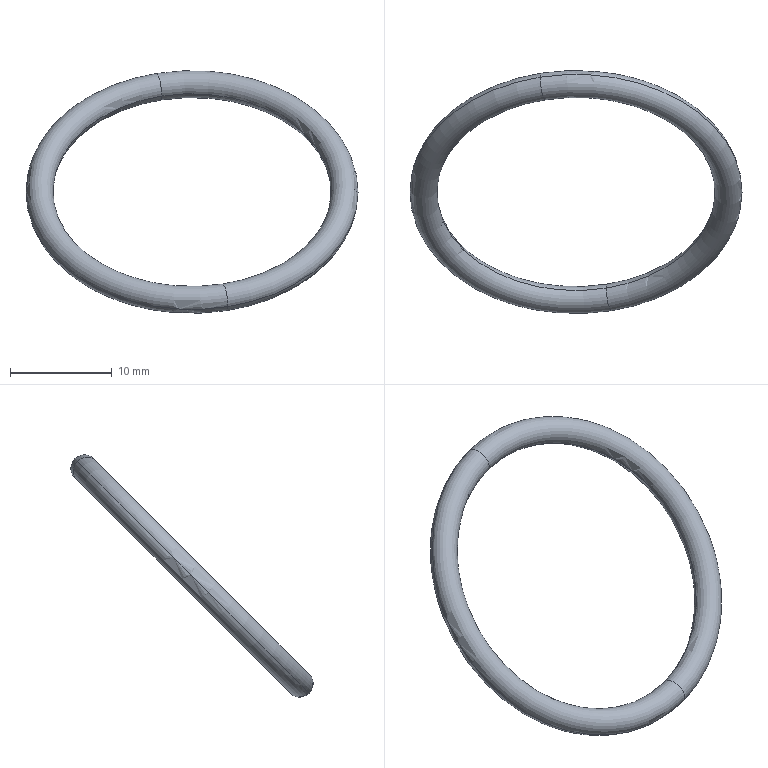Part | SolidWorks | features BaseBody 1 | 1 solid | 4 faces | box 32.65 x 23.863 x 23.863 mm | volume 519.82 mm3 | torus 4
STEP:
#1=CARTESIAN_POINT('',(247.467,236.837,-130.859));
#2=VERTEX_POINT('',#1);
#3=CARTESIAN_POINT('',(248.04,235.008,-132.688));
#4=VERTEX_POINT('',#3);
#5=CARTESIAN_POINT('',(247.753,235.922,-131.773));
#6=DIRECTION('',(0.9763,0.153,0.153));
#7=DIRECTION('',(0.1549,0.,-0.9879));
#8=AXIS2_PLACEMENT_3D('',#5,#6,#7);
#9=CIRCLE('',#8,1.325);
#10=EDGE_CURVE('',#2,#4,#9,.T.);
#11=ORIENTED_EDGE('',*,*,#10,.F.);
#12=CARTESIAN_POINT('',(254.533,214.297,-153.398));
#13=VERTEX_POINT('',#12);
#14=CARTESIAN_POINT('',(251.,225.567,-142.128));
#15=DIRECTION('',(0.,-0.7071,0.7071));
#16=DIRECTION('',(0.,-0.7071,-0.7071));
#17=AXIS2_PLACEMENT_3D('',#14,#15,#16);
#18=CIRCLE('',#17,16.325);
#19=EDGE_CURVE('',#2,#13,#18,.T.);
#20=ORIENTED_EDGE('',*,*,#19,.T.);
#21=CARTESIAN_POINT('',(253.96,216.127,-151.569));
#22=VERTEX_POINT('',#21);
#23=CARTESIAN_POINT('',(254.247,215.212,-152.484));
#24=DIRECTION('',(-0.9763,-0.153,-0.153));
#25=DIRECTION('',(-0.1549,0.,0.9879));
#26=AXIS2_PLACEMENT_3D('',#23,#24,#25);
#27=CIRCLE('',#26,1.325);
#28=EDGE_CURVE('',#13,#22,#27,.T.);
#29=ORIENTED_EDGE('',*,*,#28,.T.);
#30=CARTESIAN_POINT('',(251.,225.567,-142.128));
#31=DIRECTION('',(0.,-0.7071,0.7071));
#32=DIRECTION('',(0.,-0.7071,-0.7071));
#33=AXIS2_PLACEMENT_3D('',#30,#31,#32);
#34=CIRCLE('',#33,13.675);
#35=EDGE_CURVE('',#4,#22,#34,.T.);
#36=ORIENTED_EDGE('',*,*,#35,.F.);
#37=EDGE_LOOP('',(#11,#20,#29,#36));
#38=FACE_OUTER_BOUND('',#37,.T.);
#39=CARTESIAN_POINT('',(251.,225.567,-142.128));
#40=DIRECTION('',(0.,-0.7071,0.7071));
#41=DIRECTION('',(0.2164,-0.6903,-0.6903));
#42=AXIS2_PLACEMENT_3D('',#39,#40,#41);
#43=TOROIDAL_SURFACE('',#42,15.,1.325);
#44=ADVANCED_FACE('',(#38),#43,.T.);
#45=ORIENTED_EDGE('',*,*,#28,.F.);
#46=CARTESIAN_POINT('',(251.,225.567,-142.128));
#47=DIRECTION('',(0.,-0.7071,0.7071));
#48=DIRECTION('',(0.,-0.7071,-0.7071));
#49=AXIS2_PLACEMENT_3D('',#46,#47,#48);
#50=CIRCLE('',#49,16.325);
#51=EDGE_CURVE('',#13,#2,#50,.T.);
#52=ORIENTED_EDGE('',*,*,#51,.T.);
#53=ORIENTED_EDGE('',*,*,#10,.T.);
#54=CARTESIAN_POINT('',(251.,225.567,-142.128));
#55=DIRECTION('',(0.,-0.7071,0.7071));
#56=DIRECTION('',(0.,-0.7071,-0.7071));
#57=AXIS2_PLACEMENT_3D('',#54,#55,#56);
#58=CIRCLE('',#57,13.675);
#59=EDGE_CURVE('',#22,#4,#58,.T.);
#60=ORIENTED_EDGE('',*,*,#59,.F.);
#61=EDGE_LOOP('',(#45,#52,#53,#60));
#62=FACE_OUTER_BOUND('',#61,.T.);
#63=CARTESIAN_POINT('',(251.,225.567,-142.128));
#64=DIRECTION('',(0.,-0.7071,0.7071));
#65=DIRECTION('',(0.2164,-0.6903,-0.6903));
#66=AXIS2_PLACEMENT_3D('',#63,#64,#65);
#67=TOROIDAL_SURFACE('',#66,15.,1.325);
#68=ADVANCED_FACE('',(#62),#67,.T.);
#69=ORIENTED_EDGE('',*,*,#51,.F.);
#70=CARTESIAN_POINT('',(254.247,215.212,-152.484));
#71=DIRECTION('',(-0.9763,-0.153,-0.153));
#72=DIRECTION('',(-0.1549,0.,0.9879));
#73=AXIS2_PLACEMENT_3D('',#70,#71,#72);
#74=CIRCLE('',#73,1.325);
#75=EDGE_CURVE('',#22,#13,#74,.T.);
#76=ORIENTED_EDGE('',*,*,#75,.F.);
#77=ORIENTED_EDGE('',*,*,#59,.T.);
#78=CARTESIAN_POINT('',(247.753,235.922,-131.773));
#79=DIRECTION('',(0.9763,0.153,0.153));
#80=DIRECTION('',(0.1549,0.,-0.9879));
#81=AXIS2_PLACEMENT_3D('',#78,#79,#80);
#82=CIRCLE('',#81,1.325);
#83=EDGE_CURVE('',#4,#2,#82,.T.);
#84=ORIENTED_EDGE('',*,*,#83,.T.);
#85=EDGE_LOOP('',(#69,#76,#77,#84));
#86=FACE_OUTER_BOUND('',#85,.T.);
#87=CARTESIAN_POINT('',(251.,225.567,-142.128));
#88=DIRECTION('',(0.,-0.7071,0.7071));
#89=DIRECTION('',(0.2164,-0.6903,-0.6903));
#90=AXIS2_PLACEMENT_3D('',#87,#88,#89);
#91=TOROIDAL_SURFACE('',#90,15.,1.325);
#92=ADVANCED_FACE('',(#86),#91,.T.);
#93=ORIENTED_EDGE('',*,*,#19,.F.);
#94=ORIENTED_EDGE('',*,*,#83,.F.);
#95=ORIENTED_EDGE('',*,*,#35,.T.);
#96=ORIENTED_EDGE('',*,*,#75,.T.);
#97=EDGE_LOOP('',(#93,#94,#95,#96));
#98=FACE_OUTER_BOUND('',#97,.T.);
#99=CARTESIAN_POINT('',(251.,225.567,-142.128));
#100=DIRECTION('',(0.,-0.7071,0.7071));
#101=DIRECTION('',(0.2164,-0.6903,-0.6903));
#102=AXIS2_PLACEMENT_3D('',#99,#100,#101);
#103=TOROIDAL_SURFACE('',#102,15.,1.325);
#104=ADVANCED_FACE('',(#98),#103,.T.);
#105=CLOSED_SHELL('',(#44,#68,#92,#104));
#106=MANIFOLD_SOLID_BREP('',#105);
#107=CARTESIAN_POINT('',(0.,0.,0.));
#108=DIRECTION('',(0.,0.,1.));
#109=DIRECTION('',(1.,0.,0.));
#110=AXIS2_PLACEMENT_3D('',#107,#108,#109);
#111=(LENGTH_UNIT()NAMED_UNIT(*)SI_UNIT(.MILLI.,.METRE.));
#112=UNCERTAINTY_MEASURE_WITH_UNIT(LENGTH_MEASURE(0.00001),#111,'','');
#113=(NAMED_UNIT(*)PLANE_ANGLE_UNIT()SI_UNIT($,.RADIAN.));
#114=(NAMED_UNIT(*)SI_UNIT($,.STERADIAN.)SOLID_ANGLE_UNIT());
#115=(GEOMETRIC_REPRESENTATION_CONTEXT(3)GLOBAL_UNCERTAINTY_ASSIGNED_CONTEXT((#112))GLOBAL_UNIT_ASSIGNED_CONTEXT((#111,#113,#114))REPRESENTATION_CONTEXT('',''));
#116=ADVANCED_BREP_SHAPE_REPRESENTATION('',(#106,#110),#115);